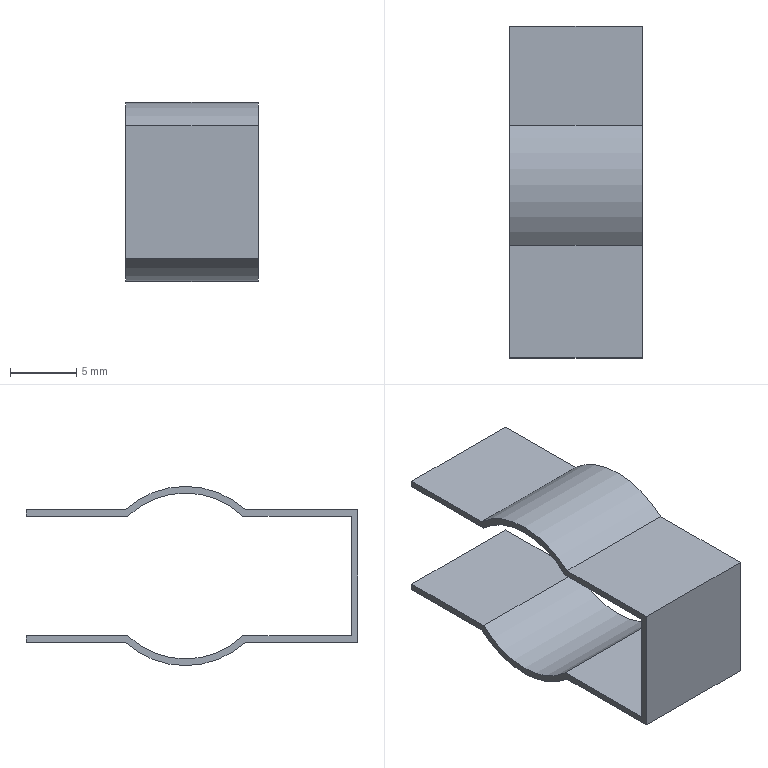Part | STEP file | 09-01 Heating tube seat | 1 solid | 18 faces | box 10 x 25 x 13.5 mm | volume 303.936 mm3 | plane 14 | cylinder 4 | commonest cylinder face diameters 12.5 x2 13.5 x2
STEP:
#1=CARTESIAN_POINT('',(0.,0.,0.));
#2=DIRECTION('',(0.,0.,1.));
#3=DIRECTION('',(1.,0.,0.));
#4=AXIS2_PLACEMENT_3D('',#1,#2,#3);
#5=CARTESIAN_POINT('',(5.,17.535,5.));
#6=VERTEX_POINT('',#5);
#7=CARTESIAN_POINT('',(5.,8.465,5.));
#8=VERTEX_POINT('',#7);
#9=CARTESIAN_POINT('',(5.,13.,0.));
#10=DIRECTION('',(1.,0.,0.));
#11=DIRECTION('',(0.,-1.,0.));
#12=AXIS2_PLACEMENT_3D('',#9,#10,#11);
#13=CIRCLE('',#12,6.75);
#14=CARTESIAN_POINT('',(5.,13.,0.));
#15=DIRECTION('',(-1.,0.,0.));
#16=DIRECTION('',(0.,-1.,0.));
#17=AXIS2_PLACEMENT_3D('',#14,#15,#16);
#18=CYLINDRICAL_SURFACE('',#17,6.75);
#19=CARTESIAN_POINT('',(6.283,0.));
#20=DIRECTION('',(-1.,0.));
#21=VECTOR('',#20,1.);
#22=LINE('',#19,#21);
#23=(GEOMETRIC_REPRESENTATION_CONTEXT(2)PARAMETRIC_REPRESENTATION_CONTEXT()REPRESENTATION_CONTEXT('',''));
#24=DEFINITIONAL_REPRESENTATION('',(#22),#23);
#25=PCURVE('',#18,#24);
#26=CARTESIAN_POINT('',(5.,0.,6.831));
#27=DIRECTION('',(1.,0.,0.));
#28=DIRECTION('',(0.,0.,-1.));
#29=AXIS2_PLACEMENT_3D('',#26,#27,#28);
#30=PLANE('',#29);
#31=CARTESIAN_POINT('',(6.831,13.));
#32=DIRECTION('',(0.,-1.));
#33=AXIS2_PLACEMENT_2D('',#31,#32);
#34=CIRCLE('',#33,6.75);
#35=(GEOMETRIC_REPRESENTATION_CONTEXT(2)PARAMETRIC_REPRESENTATION_CONTEXT()REPRESENTATION_CONTEXT('',''));
#36=DEFINITIONAL_REPRESENTATION('',(#34),#35);
#37=PCURVE('',#30,#36);
#38=SURFACE_CURVE('',#13,(#25,#37),.PCURVE_S1.);
#39=EDGE_CURVE('',#6,#8,#38,.T.);
#40=ORIENTED_EDGE('',*,*,#39,.F.);
#41=CARTESIAN_POINT('',(-5.,17.535,5.));
#42=VERTEX_POINT('',#41);
#43=CARTESIAN_POINT('',(0.,17.535,5.));
#44=DIRECTION('',(1.,0.,0.));
#45=VECTOR('',#44,1.);
#46=LINE('',#43,#45);
#47=CARTESIAN_POINT('',(2.307,5.));
#48=DIRECTION('',(0.,-1.));
#49=VECTOR('',#48,1.);
#50=LINE('',#47,#49);
#51=(GEOMETRIC_REPRESENTATION_CONTEXT(2)PARAMETRIC_REPRESENTATION_CONTEXT()REPRESENTATION_CONTEXT('',''));
#52=DEFINITIONAL_REPRESENTATION('',(#50),#51);
#53=PCURVE('',#18,#52);
#54=CARTESIAN_POINT('',(5.,17.535,5.));
#55=DIRECTION('',(0.,0.,-1.));
#56=DIRECTION('',(-1.,0.,0.));
#57=AXIS2_PLACEMENT_3D('',#54,#55,#56);
#58=PLANE('',#57);
#59=CARTESIAN_POINT('',(5.,0.));
#60=DIRECTION('',(-1.,0.));
#61=VECTOR('',#60,1.);
#62=LINE('',#59,#61);
#63=(GEOMETRIC_REPRESENTATION_CONTEXT(2)PARAMETRIC_REPRESENTATION_CONTEXT()REPRESENTATION_CONTEXT('',''));
#64=DEFINITIONAL_REPRESENTATION('',(#62),#63);
#65=PCURVE('',#58,#64);
#66=SURFACE_CURVE('',#46,(#53,#65),.PCURVE_S1.);
#67=EDGE_CURVE('',#42,#6,#66,.T.);
#68=ORIENTED_EDGE('',*,*,#67,.F.);
#69=CARTESIAN_POINT('',(-5.,8.465,5.));
#70=VERTEX_POINT('',#69);
#71=CARTESIAN_POINT('',(-5.,13.,0.));
#72=DIRECTION('',(-1.,0.,0.));
#73=DIRECTION('',(0.,-1.,0.));
#74=AXIS2_PLACEMENT_3D('',#71,#72,#73);
#75=CIRCLE('',#74,6.75);
#76=CARTESIAN_POINT('',(0.,10.));
#77=DIRECTION('',(1.,0.));
#78=VECTOR('',#77,1.);
#79=LINE('',#76,#78);
#80=(GEOMETRIC_REPRESENTATION_CONTEXT(2)PARAMETRIC_REPRESENTATION_CONTEXT()REPRESENTATION_CONTEXT('',''));
#81=DEFINITIONAL_REPRESENTATION('',(#79),#80);
#82=PCURVE('',#18,#81);
#83=CARTESIAN_POINT('',(-5.,0.,6.831));
#84=DIRECTION('',(1.,0.,0.));
#85=DIRECTION('',(0.,0.,-1.));
#86=AXIS2_PLACEMENT_3D('',#83,#84,#85);
#87=PLANE('',#86);
#88=CARTESIAN_POINT('',(6.831,6.25));
#89=CARTESIAN_POINT('',(-4.86,6.25));
#90=CARTESIAN_POINT('',(0.9853,16.375));
#91=CARTESIAN_POINT('',(6.831,26.5));
#92=CARTESIAN_POINT('',(12.677,16.375));
#93=CARTESIAN_POINT('',(18.522,6.25));
#94=CARTESIAN_POINT('',(6.831,6.25));
#95=(BOUNDED_CURVE()B_SPLINE_CURVE(2,(#88,#89,#90,#91,#92,#93,#94),.UNSPECIFIED.,.T.,.F.)B_SPLINE_CURVE_WITH_KNOTS((1,2,2,2,2,1),(-2.094,0.,2.094,4.189,6.283,8.378),.UNSPECIFIED.)CURVE()GEOMETRIC_REPRESENTATION_ITEM()RATIONAL_B_SPLINE_CURVE((1.,0.5,1.,0.5,1.,0.5,1.))REPRESENTATION_ITEM(''));
#96=(GEOMETRIC_REPRESENTATION_CONTEXT(2)PARAMETRIC_REPRESENTATION_CONTEXT()REPRESENTATION_CONTEXT('',''));
#97=DEFINITIONAL_REPRESENTATION('',(#95),#96);
#98=PCURVE('',#87,#97);
#99=SURFACE_CURVE('',#75,(#82,#98),.PCURVE_S1.);
#100=EDGE_CURVE('',#70,#42,#99,.T.);
#101=ORIENTED_EDGE('',*,*,#100,.F.);
#102=CARTESIAN_POINT('',(0.,8.465,5.));
#103=DIRECTION('',(-1.,0.,0.));
#104=VECTOR('',#103,1.);
#105=LINE('',#102,#104);
#106=CARTESIAN_POINT('',(0.8342,5.));
#107=DIRECTION('',(0.,1.));
#108=VECTOR('',#107,1.);
#109=LINE('',#106,#108);
#110=(GEOMETRIC_REPRESENTATION_CONTEXT(2)PARAMETRIC_REPRESENTATION_CONTEXT()REPRESENTATION_CONTEXT('',''));
#111=DEFINITIONAL_REPRESENTATION('',(#109),#110);
#112=PCURVE('',#18,#111);
#113=CARTESIAN_POINT('',(5.,0.,5.));
#114=DIRECTION('',(0.,0.,-1.));
#115=DIRECTION('',(-1.,0.,0.));
#116=AXIS2_PLACEMENT_3D('',#113,#114,#115);
#117=PLANE('',#116);
#118=CARTESIAN_POINT('',(5.,8.465));
#119=DIRECTION('',(1.,0.));
#120=VECTOR('',#119,1.);
#121=LINE('',#118,#120);
#122=(GEOMETRIC_REPRESENTATION_CONTEXT(2)PARAMETRIC_REPRESENTATION_CONTEXT()REPRESENTATION_CONTEXT('',''));
#123=DEFINITIONAL_REPRESENTATION('',(#121),#122);
#124=PCURVE('',#117,#123);
#125=SURFACE_CURVE('',#105,(#112,#124),.PCURVE_S1.);
#126=EDGE_CURVE('',#8,#70,#125,.T.);
#127=ORIENTED_EDGE('',*,*,#126,.F.);
#128=EDGE_LOOP('',(#40,#68,#101,#127));
#129=FACE_BOUND('',#128,.T.);
#130=ADVANCED_FACE('',(#129),#18,.T.);
#131=CARTESIAN_POINT('',(5.,25.,5.));
#132=VERTEX_POINT('',#131);
#133=CARTESIAN_POINT('',(5.,12.5,5.));
#134=DIRECTION('',(0.,-1.,0.));
#135=VECTOR('',#134,1.);
#136=LINE('',#133,#135);
#137=CARTESIAN_POINT('',(1.831,12.5));
#138=DIRECTION('',(0.,-1.));
#139=VECTOR('',#138,1.);
#140=LINE('',#137,#139);
#141=(GEOMETRIC_REPRESENTATION_CONTEXT(2)PARAMETRIC_REPRESENTATION_CONTEXT()REPRESENTATION_CONTEXT('',''));
#142=DEFINITIONAL_REPRESENTATION('',(#140),#141);
#143=PCURVE('',#30,#142);
#144=CARTESIAN_POINT('',(0.,-5.035));
#145=DIRECTION('',(0.,-1.));
#146=VECTOR('',#145,1.);
#147=LINE('',#144,#146);
#148=(GEOMETRIC_REPRESENTATION_CONTEXT(2)PARAMETRIC_REPRESENTATION_CONTEXT()REPRESENTATION_CONTEXT('',''));
#149=DEFINITIONAL_REPRESENTATION('',(#147),#148);
#150=PCURVE('',#58,#149);
#151=SURFACE_CURVE('',#136,(#143,#150),.PCURVE_S1.);
#152=EDGE_CURVE('',#132,#6,#151,.T.);
#153=ORIENTED_EDGE('',*,*,#152,.T.);
#154=ORIENTED_EDGE('',*,*,#39,.T.);
#155=CARTESIAN_POINT('',(5.,0.,5.));
#156=VERTEX_POINT('',#155);
#157=CARTESIAN_POINT('',(5.,12.5,5.));
#158=DIRECTION('',(0.,-1.,0.));
#159=VECTOR('',#158,1.);
#160=LINE('',#157,#159);
#161=CARTESIAN_POINT('',(1.831,12.5));
#162=DIRECTION('',(0.,-1.));
#163=VECTOR('',#162,1.);
#164=LINE('',#161,#163);
#165=(GEOMETRIC_REPRESENTATION_CONTEXT(2)PARAMETRIC_REPRESENTATION_CONTEXT()REPRESENTATION_CONTEXT('',''));
#166=DEFINITIONAL_REPRESENTATION('',(#164),#165);
#167=PCURVE('',#30,#166);
#168=CARTESIAN_POINT('',(0.,12.5));
#169=DIRECTION('',(0.,-1.));
#170=VECTOR('',#169,1.);
#171=LINE('',#168,#170);
#172=(GEOMETRIC_REPRESENTATION_CONTEXT(2)PARAMETRIC_REPRESENTATION_CONTEXT()REPRESENTATION_CONTEXT('',''));
#173=DEFINITIONAL_REPRESENTATION('',(#171),#172);
#174=PCURVE('',#117,#173);
#175=SURFACE_CURVE('',#160,(#167,#174),.PCURVE_S1.);
#176=EDGE_CURVE('',#8,#156,#175,.T.);
#177=ORIENTED_EDGE('',*,*,#176,.T.);
#178=CARTESIAN_POINT('',(5.,0.,-5.));
#179=VERTEX_POINT('',#178);
#180=CARTESIAN_POINT('',(5.,0.,0.));
#181=DIRECTION('',(0.,0.,-1.));
#182=VECTOR('',#181,1.);
#183=LINE('',#180,#182);
#184=CARTESIAN_POINT('',(6.831,0.));
#185=DIRECTION('',(1.,0.));
#186=VECTOR('',#185,1.);
#187=LINE('',#184,#186);
#188=(GEOMETRIC_REPRESENTATION_CONTEXT(2)PARAMETRIC_REPRESENTATION_CONTEXT()REPRESENTATION_CONTEXT('',''));
#189=DEFINITIONAL_REPRESENTATION('',(#187),#188);
#190=PCURVE('',#30,#189);
#191=CARTESIAN_POINT('',(-5.,0.,-5.));
#192=DIRECTION('',(0.,1.,0.));
#193=DIRECTION('',(0.,0.,1.));
#194=AXIS2_PLACEMENT_3D('',#191,#192,#193);
#195=PLANE('',#194);
#196=CARTESIAN_POINT('',(5.,10.));
#197=DIRECTION('',(-1.,0.));
#198=VECTOR('',#197,1.);
#199=LINE('',#196,#198);
#200=(GEOMETRIC_REPRESENTATION_CONTEXT(2)PARAMETRIC_REPRESENTATION_CONTEXT()REPRESENTATION_CONTEXT('',''));
#201=DEFINITIONAL_REPRESENTATION('',(#199),#200);
#202=PCURVE('',#195,#201);
#203=SURFACE_CURVE('',#183,(#190,#202),.PCURVE_S1.);
#204=EDGE_CURVE('',#156,#179,#203,.T.);
#205=ORIENTED_EDGE('',*,*,#204,.T.);
#206=CARTESIAN_POINT('',(5.,8.465,-5.));
#207=VERTEX_POINT('',#206);
#208=CARTESIAN_POINT('',(5.,12.5,-5.));
#209=DIRECTION('',(0.,1.,0.));
#210=VECTOR('',#209,1.);
#211=LINE('',#208,#210);
#212=CARTESIAN_POINT('',(11.831,12.5));
#213=DIRECTION('',(0.,1.));
#214=VECTOR('',#213,1.);
#215=LINE('',#212,#214);
#216=(GEOMETRIC_REPRESENTATION_CONTEXT(2)PARAMETRIC_REPRESENTATION_CONTEXT()REPRESENTATION_CONTEXT('',''));
#217=DEFINITIONAL_REPRESENTATION('',(#215),#216);
#218=PCURVE('',#30,#217);
#219=CARTESIAN_POINT('',(-5.,0.,-5.));
#220=DIRECTION('',(0.,0.,1.));
#221=DIRECTION('',(1.,0.,0.));
#222=AXIS2_PLACEMENT_3D('',#219,#220,#221);
#223=PLANE('',#222);
#224=CARTESIAN_POINT('',(10.,12.5));
#225=DIRECTION('',(0.,1.));
#226=VECTOR('',#225,1.);
#227=LINE('',#224,#226);
#228=(GEOMETRIC_REPRESENTATION_CONTEXT(2)PARAMETRIC_REPRESENTATION_CONTEXT()REPRESENTATION_CONTEXT('',''));
#229=DEFINITIONAL_REPRESENTATION('',(#227),#228);
#230=PCURVE('',#223,#229);
#231=SURFACE_CURVE('',#211,(#218,#230),.PCURVE_S1.);
#232=EDGE_CURVE('',#179,#207,#231,.T.);
#233=ORIENTED_EDGE('',*,*,#232,.T.);
#234=CARTESIAN_POINT('',(5.,17.535,-5.));
#235=VERTEX_POINT('',#234);
#236=CARTESIAN_POINT('',(5.,13.,0.));
#237=DIRECTION('',(1.,0.,0.));
#238=DIRECTION('',(0.,-1.,0.));
#239=AXIS2_PLACEMENT_3D('',#236,#237,#238);
#240=CIRCLE('',#239,6.75);
#241=CARTESIAN_POINT('',(6.831,13.));
#242=DIRECTION('',(0.,-1.));
#243=AXIS2_PLACEMENT_2D('',#241,#242);
#244=CIRCLE('',#243,6.75);
#245=(GEOMETRIC_REPRESENTATION_CONTEXT(2)PARAMETRIC_REPRESENTATION_CONTEXT()REPRESENTATION_CONTEXT('',''));
#246=DEFINITIONAL_REPRESENTATION('',(#244),#245);
#247=PCURVE('',#30,#246);
#248=CARTESIAN_POINT('',(5.,13.,0.));
#249=DIRECTION('',(-1.,0.,0.));
#250=DIRECTION('',(0.,-1.,0.));
#251=AXIS2_PLACEMENT_3D('',#248,#249,#250);
#252=CYLINDRICAL_SURFACE('',#251,6.75);
#253=CARTESIAN_POINT('',(6.283,0.));
#254=DIRECTION('',(-1.,0.));
#255=VECTOR('',#254,1.);
#256=LINE('',#253,#255);
#257=(GEOMETRIC_REPRESENTATION_CONTEXT(2)PARAMETRIC_REPRESENTATION_CONTEXT()REPRESENTATION_CONTEXT('',''));
#258=DEFINITIONAL_REPRESENTATION('',(#256),#257);
#259=PCURVE('',#252,#258);
#260=SURFACE_CURVE('',#240,(#247,#259),.PCURVE_S1.);
#261=EDGE_CURVE('',#207,#235,#260,.T.);
#262=ORIENTED_EDGE('',*,*,#261,.T.);
#263=CARTESIAN_POINT('',(5.,25.,-5.));
#264=VERTEX_POINT('',#263);
#265=CARTESIAN_POINT('',(5.,12.5,-5.));
#266=DIRECTION('',(0.,1.,0.));
#267=VECTOR('',#266,1.);
#268=LINE('',#265,#267);
#269=CARTESIAN_POINT('',(11.831,12.5));
#270=DIRECTION('',(0.,1.));
#271=VECTOR('',#270,1.);
#272=LINE('',#269,#271);
#273=(GEOMETRIC_REPRESENTATION_CONTEXT(2)PARAMETRIC_REPRESENTATION_CONTEXT()REPRESENTATION_CONTEXT('',''));
#274=DEFINITIONAL_REPRESENTATION('',(#272),#273);
#275=PCURVE('',#30,#274);
#276=CARTESIAN_POINT('',(-5.,25.,-5.));
#277=DIRECTION('',(0.,0.,1.));
#278=DIRECTION('',(0.,-1.,0.));
#279=AXIS2_PLACEMENT_3D('',#276,#277,#278);
#280=PLANE('',#279);
#281=CARTESIAN_POINT('',(12.5,10.));
#282=DIRECTION('',(-1.,0.));
#283=VECTOR('',#282,1.);
#284=LINE('',#281,#283);
#285=(GEOMETRIC_REPRESENTATION_CONTEXT(2)PARAMETRIC_REPRESENTATION_CONTEXT()REPRESENTATION_CONTEXT('',''));
#286=DEFINITIONAL_REPRESENTATION('',(#284),#285);
#287=PCURVE('',#280,#286);
#288=SURFACE_CURVE('',#268,(#275,#287),.PCURVE_S1.);
#289=EDGE_CURVE('',#235,#264,#288,.T.);
#290=ORIENTED_EDGE('',*,*,#289,.T.);
#291=CARTESIAN_POINT('',(5.,25.,-4.5));
#292=VERTEX_POINT('',#291);
#293=CARTESIAN_POINT('',(5.,25.,-4.75));
#294=DIRECTION('',(0.,0.,1.));
#295=VECTOR('',#294,1.);
#296=LINE('',#293,#295);
#297=CARTESIAN_POINT('',(11.581,25.));
#298=DIRECTION('',(-1.,0.));
#299=VECTOR('',#298,1.);
#300=LINE('',#297,#299);
#301=(GEOMETRIC_REPRESENTATION_CONTEXT(2)PARAMETRIC_REPRESENTATION_CONTEXT()REPRESENTATION_CONTEXT('',''));
#302=DEFINITIONAL_REPRESENTATION('',(#300),#301);
#303=PCURVE('',#30,#302);
#304=CARTESIAN_POINT('',(-5.,25.,-4.5));
#305=DIRECTION('',(0.,-1.,0.));
#306=DIRECTION('',(0.,0.,-1.));
#307=AXIS2_PLACEMENT_3D('',#304,#305,#306);
#308=PLANE('',#307);
#309=CARTESIAN_POINT('',(0.25,10.));
#310=DIRECTION('',(-1.,0.));
#311=VECTOR('',#310,1.);
#312=LINE('',#309,#311);
#313=(GEOMETRIC_REPRESENTATION_CONTEXT(2)PARAMETRIC_REPRESENTATION_CONTEXT()REPRESENTATION_CONTEXT('',''));
#314=DEFINITIONAL_REPRESENTATION('',(#312),#313);
#315=PCURVE('',#308,#314);
#316=SURFACE_CURVE('',#296,(#303,#315),.PCURVE_S1.);
#317=EDGE_CURVE('',#264,#292,#316,.T.);
#318=ORIENTED_EDGE('',*,*,#317,.T.);
#319=CARTESIAN_POINT('',(5.,17.337,-4.5));
#320=VERTEX_POINT('',#319);
#321=CARTESIAN_POINT('',(5.,12.5,-4.5));
#322=DIRECTION('',(0.,-1.,0.));
#323=VECTOR('',#322,1.);
#324=LINE('',#321,#323);
#325=CARTESIAN_POINT('',(11.331,12.5));
#326=DIRECTION('',(0.,-1.));
#327=VECTOR('',#326,1.);
#328=LINE('',#325,#327);
#329=(GEOMETRIC_REPRESENTATION_CONTEXT(2)PARAMETRIC_REPRESENTATION_CONTEXT()REPRESENTATION_CONTEXT('',''));
#330=DEFINITIONAL_REPRESENTATION('',(#328),#329);
#331=PCURVE('',#30,#330);
#332=CARTESIAN_POINT('',(5.,17.337,-4.5));
#333=DIRECTION('',(0.,0.,-1.));
#334=DIRECTION('',(-1.,0.,0.));
#335=AXIS2_PLACEMENT_3D('',#332,#333,#334);
#336=PLANE('',#335);
#337=CARTESIAN_POINT('',(0.,-4.837));
#338=DIRECTION('',(0.,-1.));
#339=VECTOR('',#338,1.);
#340=LINE('',#337,#339);
#341=(GEOMETRIC_REPRESENTATION_CONTEXT(2)PARAMETRIC_REPRESENTATION_CONTEXT()REPRESENTATION_CONTEXT('',''));
#342=DEFINITIONAL_REPRESENTATION('',(#340),#341);
#343=PCURVE('',#336,#342);
#344=SURFACE_CURVE('',#324,(#331,#343),.PCURVE_S1.);
#345=EDGE_CURVE('',#292,#320,#344,.T.);
#346=ORIENTED_EDGE('',*,*,#345,.T.);
#347=CARTESIAN_POINT('',(5.,8.663,-4.5));
#348=VERTEX_POINT('',#347);
#349=CARTESIAN_POINT('',(5.,13.,0.));
#350=DIRECTION('',(-1.,0.,0.));
#351=DIRECTION('',(0.,-1.,0.));
#352=AXIS2_PLACEMENT_3D('',#349,#350,#351);
#353=CIRCLE('',#352,6.25);
#354=CARTESIAN_POINT('',(6.831,6.75));
#355=CARTESIAN_POINT('',(-3.994,6.75));
#356=CARTESIAN_POINT('',(1.418,16.125));
#357=CARTESIAN_POINT('',(6.831,25.5));
#358=CARTESIAN_POINT('',(12.244,16.125));
#359=CARTESIAN_POINT('',(17.656,6.75));
#360=CARTESIAN_POINT('',(6.831,6.75));
#361=(BOUNDED_CURVE()B_SPLINE_CURVE(2,(#354,#355,#356,#357,#358,#359,#360),.UNSPECIFIED.,.T.,.F.)B_SPLINE_CURVE_WITH_KNOTS((1,2,2,2,2,1),(-2.094,0.,2.094,4.189,6.283,8.378),.UNSPECIFIED.)CURVE()GEOMETRIC_REPRESENTATION_ITEM()RATIONAL_B_SPLINE_CURVE((1.,0.5,1.,0.5,1.,0.5,1.))REPRESENTATION_ITEM(''));
#362=(GEOMETRIC_REPRESENTATION_CONTEXT(2)PARAMETRIC_REPRESENTATION_CONTEXT()REPRESENTATION_CONTEXT('',''));
#363=DEFINITIONAL_REPRESENTATION('',(#361),#362);
#364=PCURVE('',#30,#363);
#365=CARTESIAN_POINT('',(5.,13.,0.));
#366=DIRECTION('',(-1.,0.,0.));
#367=DIRECTION('',(0.,-1.,0.));
#368=AXIS2_PLACEMENT_3D('',#365,#366,#367);
#369=CYLINDRICAL_SURFACE('',#368,6.25);
#370=CARTESIAN_POINT('',(0.,0.));
#371=DIRECTION('',(1.,0.));
#372=VECTOR('',#371,1.);
#373=LINE('',#370,#372);
#374=(GEOMETRIC_REPRESENTATION_CONTEXT(2)PARAMETRIC_REPRESENTATION_CONTEXT()REPRESENTATION_CONTEXT('',''));
#375=DEFINITIONAL_REPRESENTATION('',(#373),#374);
#376=PCURVE('',#369,#375);
#377=SURFACE_CURVE('',#353,(#364,#376),.PCURVE_S1.);
#378=EDGE_CURVE('',#320,#348,#377,.T.);
#379=ORIENTED_EDGE('',*,*,#378,.T.);
#380=CARTESIAN_POINT('',(5.,0.5,-4.5));
#381=VERTEX_POINT('',#380);
#382=CARTESIAN_POINT('',(5.,12.5,-4.5));
#383=DIRECTION('',(0.,-1.,0.));
#384=VECTOR('',#383,1.);
#385=LINE('',#382,#384);
#386=CARTESIAN_POINT('',(11.331,12.5));
#387=DIRECTION('',(0.,-1.));
#388=VECTOR('',#387,1.);
#389=LINE('',#386,#388);
#390=(GEOMETRIC_REPRESENTATION_CONTEXT(2)PARAMETRIC_REPRESENTATION_CONTEXT()REPRESENTATION_CONTEXT('',''));
#391=DEFINITIONAL_REPRESENTATION('',(#389),#390);
#392=PCURVE('',#30,#391);
#393=CARTESIAN_POINT('',(-5.,0.5,-4.5));
#394=DIRECTION('',(0.,0.,-1.));
#395=DIRECTION('',(0.,1.,0.));
#396=AXIS2_PLACEMENT_3D('',#393,#394,#395);
#397=PLANE('',#396);
#398=CARTESIAN_POINT('',(12.,10.));
#399=DIRECTION('',(-1.,0.));
#400=VECTOR('',#399,1.);
#401=LINE('',#398,#400);
#402=(GEOMETRIC_REPRESENTATION_CONTEXT(2)PARAMETRIC_REPRESENTATION_CONTEXT()REPRESENTATION_CONTEXT('',''));
#403=DEFINITIONAL_REPRESENTATION('',(#401),#402);
#404=PCURVE('',#397,#403);
#405=SURFACE_CURVE('',#385,(#392,#404),.PCURVE_S1.);
#406=EDGE_CURVE('',#348,#381,#405,.T.);
#407=ORIENTED_EDGE('',*,*,#406,.T.);
#408=CARTESIAN_POINT('',(5.,0.5,4.5));
#409=VERTEX_POINT('',#408);
#410=CARTESIAN_POINT('',(5.,0.5,0.));
#411=DIRECTION('',(0.,0.,1.));
#412=VECTOR('',#411,1.);
#413=LINE('',#410,#412);
#414=CARTESIAN_POINT('',(6.831,0.5));
#415=DIRECTION('',(-1.,0.));
#416=VECTOR('',#415,1.);
#417=LINE('',#414,#416);
#418=(GEOMETRIC_REPRESENTATION_CONTEXT(2)PARAMETRIC_REPRESENTATION_CONTEXT()REPRESENTATION_CONTEXT('',''));
#419=DEFINITIONAL_REPRESENTATION('',(#417),#418);
#420=PCURVE('',#30,#419);
#421=CARTESIAN_POINT('',(-5.,0.5,4.5));
#422=DIRECTION('',(0.,-1.,0.));
#423=DIRECTION('',(0.,0.,-1.));
#424=AXIS2_PLACEMENT_3D('',#421,#422,#423);
#425=PLANE('',#424);
#426=CARTESIAN_POINT('',(4.5,10.));
#427=DIRECTION('',(-1.,0.));
#428=VECTOR('',#427,1.);
#429=LINE('',#426,#428);
#430=(GEOMETRIC_REPRESENTATION_CONTEXT(2)PARAMETRIC_REPRESENTATION_CONTEXT()REPRESENTATION_CONTEXT('',''));
#431=DEFINITIONAL_REPRESENTATION('',(#429),#430);
#432=PCURVE('',#425,#431);
#433=SURFACE_CURVE('',#413,(#420,#432),.PCURVE_S1.);
#434=EDGE_CURVE('',#381,#409,#433,.T.);
#435=ORIENTED_EDGE('',*,*,#434,.T.);
#436=CARTESIAN_POINT('',(5.,8.663,4.5));
#437=VERTEX_POINT('',#436);
#438=CARTESIAN_POINT('',(5.,12.5,4.5));
#439=DIRECTION('',(0.,1.,0.));
#440=VECTOR('',#439,1.);
#441=LINE('',#438,#440);
#442=CARTESIAN_POINT('',(2.331,12.5));
#443=DIRECTION('',(0.,1.));
#444=VECTOR('',#443,1.);
#445=LINE('',#442,#444);
#446=(GEOMETRIC_REPRESENTATION_CONTEXT(2)PARAMETRIC_REPRESENTATION_CONTEXT()REPRESENTATION_CONTEXT('',''));
#447=DEFINITIONAL_REPRESENTATION('',(#445),#446);
#448=PCURVE('',#30,#447);
#449=CARTESIAN_POINT('',(-5.,0.5,4.5));
#450=DIRECTION('',(0.,0.,1.));
#451=DIRECTION('',(1.,0.,0.));
#452=AXIS2_PLACEMENT_3D('',#449,#450,#451);
#453=PLANE('',#452);
#454=CARTESIAN_POINT('',(10.,12.));
#455=DIRECTION('',(0.,1.));
#456=VECTOR('',#455,1.);
#457=LINE('',#454,#456);
#458=(GEOMETRIC_REPRESENTATION_CONTEXT(2)PARAMETRIC_REPRESENTATION_CONTEXT()REPRESENTATION_CONTEXT('',''));
#459=DEFINITIONAL_REPRESENTATION('',(#457),#458);
#460=PCURVE('',#453,#459);
#461=SURFACE_CURVE('',#441,(#448,#460),.PCURVE_S1.);
#462=EDGE_CURVE('',#409,#437,#461,.T.);
#463=ORIENTED_EDGE('',*,*,#462,.T.);
#464=CARTESIAN_POINT('',(5.,17.337,4.5));
#465=VERTEX_POINT('',#464);
#466=CARTESIAN_POINT('',(5.,13.,0.));
#467=DIRECTION('',(-1.,0.,0.));
#468=DIRECTION('',(0.,-1.,0.));
#469=AXIS2_PLACEMENT_3D('',#466,#467,#468);
#470=CIRCLE('',#469,6.25);
#471=CARTESIAN_POINT('',(6.831,6.75));
#472=CARTESIAN_POINT('',(-3.994,6.75));
#473=CARTESIAN_POINT('',(1.418,16.125));
#474=CARTESIAN_POINT('',(6.831,25.5));
#475=CARTESIAN_POINT('',(12.244,16.125));
#476=CARTESIAN_POINT('',(17.656,6.75));
#477=CARTESIAN_POINT('',(6.831,6.75));
#478=(BOUNDED_CURVE()B_SPLINE_CURVE(2,(#471,#472,#473,#474,#475,#476,#477),.UNSPECIFIED.,.T.,.F.)B_SPLINE_CURVE_WITH_KNOTS((1,2,2,2,2,1),(-2.094,0.,2.094,4.189,6.283,8.378),.UNSPECIFIED.)CURVE()GEOMETRIC_REPRESENTATION_ITEM()RATIONAL_B_SPLINE_CURVE((1.,0.5,1.,0.5,1.,0.5,1.))REPRESENTATION_ITEM(''));
#479=(GEOMETRIC_REPRESENTATION_CONTEXT(2)PARAMETRIC_REPRESENTATION_CONTEXT()REPRESENTATION_CONTEXT('',''));
#480=DEFINITIONAL_REPRESENTATION('',(#478),#479);
#481=PCURVE('',#30,#480);
#482=CARTESIAN_POINT('',(5.,13.,0.));
#483=DIRECTION('',(-1.,0.,0.));
#484=DIRECTION('',(0.,-1.,0.));
#485=AXIS2_PLACEMENT_3D('',#482,#483,#484);
#486=CYLINDRICAL_SURFACE('',#485,6.25);
#487=CARTESIAN_POINT('',(0.,0.));
#488=DIRECTION('',(1.,0.));
#489=VECTOR('',#488,1.);
#490=LINE('',#487,#489);
#491=(GEOMETRIC_REPRESENTATION_CONTEXT(2)PARAMETRIC_REPRESENTATION_CONTEXT()REPRESENTATION_CONTEXT('',''));
#492=DEFINITIONAL_REPRESENTATION('',(#490),#491);
#493=PCURVE('',#486,#492);
#494=SURFACE_CURVE('',#470,(#481,#493),.PCURVE_S1.);
#495=EDGE_CURVE('',#437,#465,#494,.T.);
#496=ORIENTED_EDGE('',*,*,#495,.T.);
#497=CARTESIAN_POINT('',(5.,25.,4.5));
#498=VERTEX_POINT('',#497);
#499=CARTESIAN_POINT('',(5.,12.5,4.5));
#500=DIRECTION('',(0.,1.,0.));
#501=VECTOR('',#500,1.);
#502=LINE('',#499,#501);
#503=CARTESIAN_POINT('',(2.331,12.5));
#504=DIRECTION('',(0.,1.));
#505=VECTOR('',#504,1.);
#506=LINE('',#503,#505);
#507=(GEOMETRIC_REPRESENTATION_CONTEXT(2)PARAMETRIC_REPRESENTATION_CONTEXT()REPRESENTATION_CONTEXT('',''));
#508=DEFINITIONAL_REPRESENTATION('',(#506),#507);
#509=PCURVE('',#30,#508);
#510=CARTESIAN_POINT('',(-5.,17.337,4.5));
#511=DIRECTION('',(0.,0.,1.));
#512=DIRECTION('',(1.,0.,0.));
#513=AXIS2_PLACEMENT_3D('',#510,#511,#512);
#514=PLANE('',#513);
#515=CARTESIAN_POINT('',(10.,-4.837));
#516=DIRECTION('',(0.,1.));
#517=VECTOR('',#516,1.);
#518=LINE('',#515,#517);
#519=(GEOMETRIC_REPRESENTATION_CONTEXT(2)PARAMETRIC_REPRESENTATION_CONTEXT()REPRESENTATION_CONTEXT('',''));
#520=DEFINITIONAL_REPRESENTATION('',(#518),#519);
#521=PCURVE('',#514,#520);
#522=SURFACE_CURVE('',#502,(#509,#521),.PCURVE_S1.);
#523=EDGE_CURVE('',#465,#498,#522,.T.);
#524=ORIENTED_EDGE('',*,*,#523,.T.);
#525=CARTESIAN_POINT('',(5.,25.,4.75));
#526=DIRECTION('',(0.,0.,1.));
#527=VECTOR('',#526,1.);
#528=LINE('',#525,#527);
#529=CARTESIAN_POINT('',(2.081,25.));
#530=DIRECTION('',(-1.,0.));
#531=VECTOR('',#530,1.);
#532=LINE('',#529,#531);
#533=(GEOMETRIC_REPRESENTATION_CONTEXT(2)PARAMETRIC_REPRESENTATION_CONTEXT()REPRESENTATION_CONTEXT('',''));
#534=DEFINITIONAL_REPRESENTATION('',(#532),#533);
#535=PCURVE('',#30,#534);
#536=CARTESIAN_POINT('',(-5.,25.,5.));
#537=DIRECTION('',(0.,-1.,0.));
#538=DIRECTION('',(0.,0.,-1.));
#539=AXIS2_PLACEMENT_3D('',#536,#537,#538);
#540=PLANE('',#539);
#541=CARTESIAN_POINT('',(0.25,10.));
#542=DIRECTION('',(-1.,0.));
#543=VECTOR('',#542,1.);
#544=LINE('',#541,#543);
#545=(GEOMETRIC_REPRESENTATION_CONTEXT(2)PARAMETRIC_REPRESENTATION_CONTEXT()REPRESENTATION_CONTEXT('',''));
#546=DEFINITIONAL_REPRESENTATION('',(#544),#545);
#547=PCURVE('',#540,#546);
#548=SURFACE_CURVE('',#528,(#535,#547),.PCURVE_S1.);
#549=EDGE_CURVE('',#498,#132,#548,.T.);
#550=ORIENTED_EDGE('',*,*,#549,.T.);
#551=EDGE_LOOP('',(#153,#154,#177,#205,#233,#262,#290,#318,#346,#379,#407,#435,#463,#496,#524,#550));
#552=FACE_BOUND('',#551,.T.);
#553=ADVANCED_FACE('',(#552),#30,.T.);
#554=ORIENTED_EDGE('',*,*,#100,.T.);
#555=CARTESIAN_POINT('',(-5.,25.,5.));
#556=VERTEX_POINT('',#555);
#557=CARTESIAN_POINT('',(-5.,12.5,5.));
#558=DIRECTION('',(0.,-1.,0.));
#559=VECTOR('',#558,1.);
#560=LINE('',#557,#559);
#561=CARTESIAN_POINT('',(1.831,12.5));
#562=DIRECTION('',(0.,-1.));
#563=VECTOR('',#562,1.);
#564=LINE('',#561,#563);
#565=(GEOMETRIC_REPRESENTATION_CONTEXT(2)PARAMETRIC_REPRESENTATION_CONTEXT()REPRESENTATION_CONTEXT('',''));
#566=DEFINITIONAL_REPRESENTATION('',(#564),#565);
#567=PCURVE('',#87,#566);
#568=CARTESIAN_POINT('',(10.,-5.035));
#569=DIRECTION('',(0.,-1.));
#570=VECTOR('',#569,1.);
#571=LINE('',#568,#570);
#572=(GEOMETRIC_REPRESENTATION_CONTEXT(2)PARAMETRIC_REPRESENTATION_CONTEXT()REPRESENTATION_CONTEXT('',''));
#573=DEFINITIONAL_REPRESENTATION('',(#571),#572);
#574=PCURVE('',#58,#573);
#575=SURFACE_CURVE('',#560,(#567,#574),.PCURVE_S1.);
#576=EDGE_CURVE('',#556,#42,#575,.T.);
#577=ORIENTED_EDGE('',*,*,#576,.F.);
#578=CARTESIAN_POINT('',(-5.,25.,4.5));
#579=VERTEX_POINT('',#578);
#580=CARTESIAN_POINT('',(-5.,25.,4.75));
#581=DIRECTION('',(0.,0.,-1.));
#582=VECTOR('',#581,1.);
#583=LINE('',#580,#582);
#584=CARTESIAN_POINT('',(2.081,25.));
#585=DIRECTION('',(1.,0.));
#586=VECTOR('',#585,1.);
#587=LINE('',#584,#586);
#588=(GEOMETRIC_REPRESENTATION_CONTEXT(2)PARAMETRIC_REPRESENTATION_CONTEXT()REPRESENTATION_CONTEXT('',''));
#589=DEFINITIONAL_REPRESENTATION('',(#587),#588);
#590=PCURVE('',#87,#589);
#591=CARTESIAN_POINT('',(0.25,0.));
#592=DIRECTION('',(1.,0.));
#593=VECTOR('',#592,1.);
#594=LINE('',#591,#593);
#595=(GEOMETRIC_REPRESENTATION_CONTEXT(2)PARAMETRIC_REPRESENTATION_CONTEXT()REPRESENTATION_CONTEXT('',''));
#596=DEFINITIONAL_REPRESENTATION('',(#594),#595);
#597=PCURVE('',#540,#596);
#598=SURFACE_CURVE('',#583,(#590,#597),.PCURVE_S1.);
#599=EDGE_CURVE('',#556,#579,#598,.T.);
#600=ORIENTED_EDGE('',*,*,#599,.T.);
#601=CARTESIAN_POINT('',(-5.,17.337,4.5));
#602=VERTEX_POINT('',#601);
#603=CARTESIAN_POINT('',(-5.,12.5,4.5));
#604=DIRECTION('',(0.,1.,0.));
#605=VECTOR('',#604,1.);
#606=LINE('',#603,#605);
#607=CARTESIAN_POINT('',(2.331,12.5));
#608=DIRECTION('',(0.,1.));
#609=VECTOR('',#608,1.);
#610=LINE('',#607,#609);
#611=(GEOMETRIC_REPRESENTATION_CONTEXT(2)PARAMETRIC_REPRESENTATION_CONTEXT()REPRESENTATION_CONTEXT('',''));
#612=DEFINITIONAL_REPRESENTATION('',(#610),#611);
#613=PCURVE('',#87,#612);
#614=CARTESIAN_POINT('',(0.,-4.837));
#615=DIRECTION('',(0.,1.));
#616=VECTOR('',#615,1.);
#617=LINE('',#614,#616);
#618=(GEOMETRIC_REPRESENTATION_CONTEXT(2)PARAMETRIC_REPRESENTATION_CONTEXT()REPRESENTATION_CONTEXT('',''));
#619=DEFINITIONAL_REPRESENTATION('',(#617),#618);
#620=PCURVE('',#514,#619);
#621=SURFACE_CURVE('',#606,(#613,#620),.PCURVE_S1.);
#622=EDGE_CURVE('',#602,#579,#621,.T.);
#623=ORIENTED_EDGE('',*,*,#622,.F.);
#624=CARTESIAN_POINT('',(-5.,8.663,4.5));
#625=VERTEX_POINT('',#624);
#626=CARTESIAN_POINT('',(-5.,13.,0.));
#627=DIRECTION('',(-1.,0.,0.));
#628=DIRECTION('',(0.,-1.,0.));
#629=AXIS2_PLACEMENT_3D('',#626,#627,#628);
#630=CIRCLE('',#629,6.25);
#631=CARTESIAN_POINT('',(6.831,6.75));
#632=CARTESIAN_POINT('',(-3.994,6.75));
#633=CARTESIAN_POINT('',(1.418,16.125));
#634=CARTESIAN_POINT('',(6.831,25.5));
#635=CARTESIAN_POINT('',(12.244,16.125));
#636=CARTESIAN_POINT('',(17.656,6.75));
#637=CARTESIAN_POINT('',(6.831,6.75));
#638=(BOUNDED_CURVE()B_SPLINE_CURVE(2,(#631,#632,#633,#634,#635,#636,#637),.UNSPECIFIED.,.T.,.F.)B_SPLINE_CURVE_WITH_KNOTS((1,2,2,2,2,1),(-2.094,0.,2.094,4.189,6.283,8.378),.UNSPECIFIED.)CURVE()GEOMETRIC_REPRESENTATION_ITEM()RATIONAL_B_SPLINE_CURVE((1.,0.5,1.,0.5,1.,0.5,1.))REPRESENTATION_ITEM(''));
#639=(GEOMETRIC_REPRESENTATION_CONTEXT(2)PARAMETRIC_REPRESENTATION_CONTEXT()REPRESENTATION_CONTEXT('',''));
#640=DEFINITIONAL_REPRESENTATION('',(#638),#639);
#641=PCURVE('',#87,#640);
#642=CARTESIAN_POINT('',(0.,10.));
#643=DIRECTION('',(1.,0.));
#644=VECTOR('',#643,1.);
#645=LINE('',#642,#644);
#646=(GEOMETRIC_REPRESENTATION_CONTEXT(2)PARAMETRIC_REPRESENTATION_CONTEXT()REPRESENTATION_CONTEXT('',''));
#647=DEFINITIONAL_REPRESENTATION('',(#645),#646);
#648=PCURVE('',#486,#647);
#649=SURFACE_CURVE('',#630,(#641,#648),.PCURVE_S1.);
#650=EDGE_CURVE('',#625,#602,#649,.T.);
#651=ORIENTED_EDGE('',*,*,#650,.F.);
#652=CARTESIAN_POINT('',(-5.,0.5,4.5));
#653=VERTEX_POINT('',#652);
#654=CARTESIAN_POINT('',(-5.,12.5,4.5));
#655=DIRECTION('',(0.,1.,0.));
#656=VECTOR('',#655,1.);
#657=LINE('',#654,#656);
#658=CARTESIAN_POINT('',(2.331,12.5));
#659=DIRECTION('',(0.,1.));
#660=VECTOR('',#659,1.);
#661=LINE('',#658,#660);
#662=(GEOMETRIC_REPRESENTATION_CONTEXT(2)PARAMETRIC_REPRESENTATION_CONTEXT()REPRESENTATION_CONTEXT('',''));
#663=DEFINITIONAL_REPRESENTATION('',(#661),#662);
#664=PCURVE('',#87,#663);
#665=CARTESIAN_POINT('',(0.,12.));
#666=DIRECTION('',(0.,1.));
#667=VECTOR('',#666,1.);
#668=LINE('',#665,#667);
#669=(GEOMETRIC_REPRESENTATION_CONTEXT(2)PARAMETRIC_REPRESENTATION_CONTEXT()REPRESENTATION_CONTEXT('',''));
#670=DEFINITIONAL_REPRESENTATION('',(#668),#669);
#671=PCURVE('',#453,#670);
#672=SURFACE_CURVE('',#657,(#664,#671),.PCURVE_S1.);
#673=EDGE_CURVE('',#653,#625,#672,.T.);
#674=ORIENTED_EDGE('',*,*,#673,.F.);
#675=CARTESIAN_POINT('',(-5.,0.5,-4.5));
#676=VERTEX_POINT('',#675);
#677=CARTESIAN_POINT('',(-5.,0.5,0.));
#678=DIRECTION('',(0.,0.,1.));
#679=VECTOR('',#678,1.);
#680=LINE('',#677,#679);
#681=CARTESIAN_POINT('',(6.831,0.5));
#682=DIRECTION('',(-1.,0.));
#683=VECTOR('',#682,1.);
#684=LINE('',#681,#683);
#685=(GEOMETRIC_REPRESENTATION_CONTEXT(2)PARAMETRIC_REPRESENTATION_CONTEXT()REPRESENTATION_CONTEXT('',''));
#686=DEFINITIONAL_REPRESENTATION('',(#684),#685);
#687=PCURVE('',#87,#686);
#688=CARTESIAN_POINT('',(4.5,0.));
#689=DIRECTION('',(-1.,0.));
#690=VECTOR('',#689,1.);
#691=LINE('',#688,#690);
#692=(GEOMETRIC_REPRESENTATION_CONTEXT(2)PARAMETRIC_REPRESENTATION_CONTEXT()REPRESENTATION_CONTEXT('',''));
#693=DEFINITIONAL_REPRESENTATION('',(#691),#692);
#694=PCURVE('',#425,#693);
#695=SURFACE_CURVE('',#680,(#687,#694),.PCURVE_S1.);
#696=EDGE_CURVE('',#676,#653,#695,.T.);
#697=ORIENTED_EDGE('',*,*,#696,.F.);
#698=CARTESIAN_POINT('',(-5.,8.663,-4.5));
#699=VERTEX_POINT('',#698);
#700=CARTESIAN_POINT('',(-5.,12.5,-4.5));
#701=DIRECTION('',(0.,-1.,0.));
#702=VECTOR('',#701,1.);
#703=LINE('',#700,#702);
#704=CARTESIAN_POINT('',(11.331,12.5));
#705=DIRECTION('',(0.,-1.));
#706=VECTOR('',#705,1.);
#707=LINE('',#704,#706);
#708=(GEOMETRIC_REPRESENTATION_CONTEXT(2)PARAMETRIC_REPRESENTATION_CONTEXT()REPRESENTATION_CONTEXT('',''));
#709=DEFINITIONAL_REPRESENTATION('',(#707),#708);
#710=PCURVE('',#87,#709);
#711=CARTESIAN_POINT('',(12.,0.));
#712=DIRECTION('',(-1.,0.));
#713=VECTOR('',#712,1.);
#714=LINE('',#711,#713);
#715=(GEOMETRIC_REPRESENTATION_CONTEXT(2)PARAMETRIC_REPRESENTATION_CONTEXT()REPRESENTATION_CONTEXT('',''));
#716=DEFINITIONAL_REPRESENTATION('',(#714),#715);
#717=PCURVE('',#397,#716);
#718=SURFACE_CURVE('',#703,(#710,#717),.PCURVE_S1.);
#719=EDGE_CURVE('',#699,#676,#718,.T.);
#720=ORIENTED_EDGE('',*,*,#719,.F.);
#721=CARTESIAN_POINT('',(-5.,17.337,-4.5));
#722=VERTEX_POINT('',#721);
#723=CARTESIAN_POINT('',(-5.,13.,0.));
#724=DIRECTION('',(-1.,0.,0.));
#725=DIRECTION('',(0.,-1.,0.));
#726=AXIS2_PLACEMENT_3D('',#723,#724,#725);
#727=CIRCLE('',#726,6.25);
#728=CARTESIAN_POINT('',(6.831,6.75));
#729=CARTESIAN_POINT('',(-3.994,6.75));
#730=CARTESIAN_POINT('',(1.418,16.125));
#731=CARTESIAN_POINT('',(6.831,25.5));
#732=CARTESIAN_POINT('',(12.244,16.125));
#733=CARTESIAN_POINT('',(17.656,6.75));
#734=CARTESIAN_POINT('',(6.831,6.75));
#735=(BOUNDED_CURVE()B_SPLINE_CURVE(2,(#728,#729,#730,#731,#732,#733,#734),.UNSPECIFIED.,.T.,.F.)B_SPLINE_CURVE_WITH_KNOTS((1,2,2,2,2,1),(-2.094,0.,2.094,4.189,6.283,8.378),.UNSPECIFIED.)CURVE()GEOMETRIC_REPRESENTATION_ITEM()RATIONAL_B_SPLINE_CURVE((1.,0.5,1.,0.5,1.,0.5,1.))REPRESENTATION_ITEM(''));
#736=(GEOMETRIC_REPRESENTATION_CONTEXT(2)PARAMETRIC_REPRESENTATION_CONTEXT()REPRESENTATION_CONTEXT('',''));
#737=DEFINITIONAL_REPRESENTATION('',(#735),#736);
#738=PCURVE('',#87,#737);
#739=CARTESIAN_POINT('',(0.,10.));
#740=DIRECTION('',(1.,0.));
#741=VECTOR('',#740,1.);
#742=LINE('',#739,#741);
#743=(GEOMETRIC_REPRESENTATION_CONTEXT(2)PARAMETRIC_REPRESENTATION_CONTEXT()REPRESENTATION_CONTEXT('',''));
#744=DEFINITIONAL_REPRESENTATION('',(#742),#743);
#745=PCURVE('',#369,#744);
#746=SURFACE_CURVE('',#727,(#738,#745),.PCURVE_S1.);
#747=EDGE_CURVE('',#722,#699,#746,.T.);
#748=ORIENTED_EDGE('',*,*,#747,.F.);
#749=CARTESIAN_POINT('',(-5.,25.,-4.5));
#750=VERTEX_POINT('',#749);
#751=CARTESIAN_POINT('',(-5.,12.5,-4.5));
#752=DIRECTION('',(0.,-1.,0.));
#753=VECTOR('',#752,1.);
#754=LINE('',#751,#753);
#755=CARTESIAN_POINT('',(11.331,12.5));
#756=DIRECTION('',(0.,-1.));
#757=VECTOR('',#756,1.);
#758=LINE('',#755,#757);
#759=(GEOMETRIC_REPRESENTATION_CONTEXT(2)PARAMETRIC_REPRESENTATION_CONTEXT()REPRESENTATION_CONTEXT('',''));
#760=DEFINITIONAL_REPRESENTATION('',(#758),#759);
#761=PCURVE('',#87,#760);
#762=CARTESIAN_POINT('',(10.,-4.837));
#763=DIRECTION('',(0.,-1.));
#764=VECTOR('',#763,1.);
#765=LINE('',#762,#764);
#766=(GEOMETRIC_REPRESENTATION_CONTEXT(2)PARAMETRIC_REPRESENTATION_CONTEXT()REPRESENTATION_CONTEXT('',''));
#767=DEFINITIONAL_REPRESENTATION('',(#765),#766);
#768=PCURVE('',#336,#767);
#769=SURFACE_CURVE('',#754,(#761,#768),.PCURVE_S1.);
#770=EDGE_CURVE('',#750,#722,#769,.T.);
#771=ORIENTED_EDGE('',*,*,#770,.F.);
#772=CARTESIAN_POINT('',(-5.,25.,-5.));
#773=VERTEX_POINT('',#772);
#774=CARTESIAN_POINT('',(-5.,25.,-4.75));
#775=DIRECTION('',(0.,0.,-1.));
#776=VECTOR('',#775,1.);
#777=LINE('',#774,#776);
#778=CARTESIAN_POINT('',(11.581,25.));
#779=DIRECTION('',(1.,0.));
#780=VECTOR('',#779,1.);
#781=LINE('',#778,#780);
#782=(GEOMETRIC_REPRESENTATION_CONTEXT(2)PARAMETRIC_REPRESENTATION_CONTEXT()REPRESENTATION_CONTEXT('',''));
#783=DEFINITIONAL_REPRESENTATION('',(#781),#782);
#784=PCURVE('',#87,#783);
#785=CARTESIAN_POINT('',(0.25,0.));
#786=DIRECTION('',(1.,0.));
#787=VECTOR('',#786,1.);
#788=LINE('',#785,#787);
#789=(GEOMETRIC_REPRESENTATION_CONTEXT(2)PARAMETRIC_REPRESENTATION_CONTEXT()REPRESENTATION_CONTEXT('',''));
#790=DEFINITIONAL_REPRESENTATION('',(#788),#789);
#791=PCURVE('',#308,#790);
#792=SURFACE_CURVE('',#777,(#784,#791),.PCURVE_S1.);
#793=EDGE_CURVE('',#750,#773,#792,.T.);
#794=ORIENTED_EDGE('',*,*,#793,.T.);
#795=CARTESIAN_POINT('',(-5.,17.535,-5.));
#796=VERTEX_POINT('',#795);
#797=CARTESIAN_POINT('',(-5.,12.5,-5.));
#798=DIRECTION('',(0.,1.,0.));
#799=VECTOR('',#798,1.);
#800=LINE('',#797,#799);
#801=CARTESIAN_POINT('',(11.831,12.5));
#802=DIRECTION('',(0.,1.));
#803=VECTOR('',#802,1.);
#804=LINE('',#801,#803);
#805=(GEOMETRIC_REPRESENTATION_CONTEXT(2)PARAMETRIC_REPRESENTATION_CONTEXT()REPRESENTATION_CONTEXT('',''));
#806=DEFINITIONAL_REPRESENTATION('',(#804),#805);
#807=PCURVE('',#87,#806);
#808=CARTESIAN_POINT('',(12.5,0.));
#809=DIRECTION('',(-1.,0.));
#810=VECTOR('',#809,1.);
#811=LINE('',#808,#810);
#812=(GEOMETRIC_REPRESENTATION_CONTEXT(2)PARAMETRIC_REPRESENTATION_CONTEXT()REPRESENTATION_CONTEXT('',''));
#813=DEFINITIONAL_REPRESENTATION('',(#811),#812);
#814=PCURVE('',#280,#813);
#815=SURFACE_CURVE('',#800,(#807,#814),.PCURVE_S1.);
#816=EDGE_CURVE('',#796,#773,#815,.T.);
#817=ORIENTED_EDGE('',*,*,#816,.F.);
#818=CARTESIAN_POINT('',(-5.,8.465,-5.));
#819=VERTEX_POINT('',#818);
#820=CARTESIAN_POINT('',(-5.,13.,0.));
#821=DIRECTION('',(1.,0.,0.));
#822=DIRECTION('',(0.,-1.,0.));
#823=AXIS2_PLACEMENT_3D('',#820,#821,#822);
#824=CIRCLE('',#823,6.75);
#825=CARTESIAN_POINT('',(6.831,13.));
#826=DIRECTION('',(0.,-1.));
#827=AXIS2_PLACEMENT_2D('',#825,#826);
#828=CIRCLE('',#827,6.75);
#829=(GEOMETRIC_REPRESENTATION_CONTEXT(2)PARAMETRIC_REPRESENTATION_CONTEXT()REPRESENTATION_CONTEXT('',''));
#830=DEFINITIONAL_REPRESENTATION('',(#828),#829);
#831=PCURVE('',#87,#830);
#832=CARTESIAN_POINT('',(6.283,10.));
#833=DIRECTION('',(-1.,0.));
#834=VECTOR('',#833,1.);
#835=LINE('',#832,#834);
#836=(GEOMETRIC_REPRESENTATION_CONTEXT(2)PARAMETRIC_REPRESENTATION_CONTEXT()REPRESENTATION_CONTEXT('',''));
#837=DEFINITIONAL_REPRESENTATION('',(#835),#836);
#838=PCURVE('',#252,#837);
#839=SURFACE_CURVE('',#824,(#831,#838),.PCURVE_S1.);
#840=EDGE_CURVE('',#819,#796,#839,.T.);
#841=ORIENTED_EDGE('',*,*,#840,.F.);
#842=CARTESIAN_POINT('',(-5.,0.,-5.));
#843=VERTEX_POINT('',#842);
#844=CARTESIAN_POINT('',(-5.,12.5,-5.));
#845=DIRECTION('',(0.,1.,0.));
#846=VECTOR('',#845,1.);
#847=LINE('',#844,#846);
#848=CARTESIAN_POINT('',(11.831,12.5));
#849=DIRECTION('',(0.,1.));
#850=VECTOR('',#849,1.);
#851=LINE('',#848,#850);
#852=(GEOMETRIC_REPRESENTATION_CONTEXT(2)PARAMETRIC_REPRESENTATION_CONTEXT()REPRESENTATION_CONTEXT('',''));
#853=DEFINITIONAL_REPRESENTATION('',(#851),#852);
#854=PCURVE('',#87,#853);
#855=CARTESIAN_POINT('',(0.,12.5));
#856=DIRECTION('',(0.,1.));
#857=VECTOR('',#856,1.);
#858=LINE('',#855,#857);
#859=(GEOMETRIC_REPRESENTATION_CONTEXT(2)PARAMETRIC_REPRESENTATION_CONTEXT()REPRESENTATION_CONTEXT('',''));
#860=DEFINITIONAL_REPRESENTATION('',(#858),#859);
#861=PCURVE('',#223,#860);
#862=SURFACE_CURVE('',#847,(#854,#861),.PCURVE_S1.);
#863=EDGE_CURVE('',#843,#819,#862,.T.);
#864=ORIENTED_EDGE('',*,*,#863,.F.);
#865=CARTESIAN_POINT('',(-5.,0.,5.));
#866=VERTEX_POINT('',#865);
#867=CARTESIAN_POINT('',(-5.,0.,0.));
#868=DIRECTION('',(0.,0.,-1.));
#869=VECTOR('',#868,1.);
#870=LINE('',#867,#869);
#871=CARTESIAN_POINT('',(6.831,0.));
#872=DIRECTION('',(1.,0.));
#873=VECTOR('',#872,1.);
#874=LINE('',#871,#873);
#875=(GEOMETRIC_REPRESENTATION_CONTEXT(2)PARAMETRIC_REPRESENTATION_CONTEXT()REPRESENTATION_CONTEXT('',''));
#876=DEFINITIONAL_REPRESENTATION('',(#874),#875);
#877=PCURVE('',#87,#876);
#878=CARTESIAN_POINT('',(5.,0.));
#879=DIRECTION('',(-1.,0.));
#880=VECTOR('',#879,1.);
#881=LINE('',#878,#880);
#882=(GEOMETRIC_REPRESENTATION_CONTEXT(2)PARAMETRIC_REPRESENTATION_CONTEXT()REPRESENTATION_CONTEXT('',''));
#883=DEFINITIONAL_REPRESENTATION('',(#881),#882);
#884=PCURVE('',#195,#883);
#885=SURFACE_CURVE('',#870,(#877,#884),.PCURVE_S1.);
#886=EDGE_CURVE('',#866,#843,#885,.T.);
#887=ORIENTED_EDGE('',*,*,#886,.F.);
#888=CARTESIAN_POINT('',(-5.,12.5,5.));
#889=DIRECTION('',(0.,-1.,0.));
#890=VECTOR('',#889,1.);
#891=LINE('',#888,#890);
#892=CARTESIAN_POINT('',(1.831,12.5));
#893=DIRECTION('',(0.,-1.));
#894=VECTOR('',#893,1.);
#895=LINE('',#892,#894);
#896=(GEOMETRIC_REPRESENTATION_CONTEXT(2)PARAMETRIC_REPRESENTATION_CONTEXT()REPRESENTATION_CONTEXT('',''));
#897=DEFINITIONAL_REPRESENTATION('',(#895),#896);
#898=PCURVE('',#87,#897);
#899=CARTESIAN_POINT('',(10.,12.5));
#900=DIRECTION('',(0.,-1.));
#901=VECTOR('',#900,1.);
#902=LINE('',#899,#901);
#903=(GEOMETRIC_REPRESENTATION_CONTEXT(2)PARAMETRIC_REPRESENTATION_CONTEXT()REPRESENTATION_CONTEXT('',''));
#904=DEFINITIONAL_REPRESENTATION('',(#902),#903);
#905=PCURVE('',#117,#904);
#906=SURFACE_CURVE('',#891,(#898,#905),.PCURVE_S1.);
#907=EDGE_CURVE('',#70,#866,#906,.T.);
#908=ORIENTED_EDGE('',*,*,#907,.F.);
#909=EDGE_LOOP('',(#554,#577,#600,#623,#651,#674,#697,#720,#748,#771,#794,#817,#841,#864,#887,#908));
#910=FACE_BOUND('',#909,.T.);
#911=ADVANCED_FACE('',(#910),#87,.F.);
#912=CARTESIAN_POINT('',(0.,0.,5.));
#913=DIRECTION('',(-1.,0.,0.));
#914=VECTOR('',#913,1.);
#915=LINE('',#912,#914);
#916=CARTESIAN_POINT('',(5.,0.));
#917=DIRECTION('',(1.,0.));
#918=VECTOR('',#917,1.);
#919=LINE('',#916,#918);
#920=(GEOMETRIC_REPRESENTATION_CONTEXT(2)PARAMETRIC_REPRESENTATION_CONTEXT()REPRESENTATION_CONTEXT('',''));
#921=DEFINITIONAL_REPRESENTATION('',(#919),#920);
#922=PCURVE('',#117,#921);
#923=CARTESIAN_POINT('',(10.,5.));
#924=DIRECTION('',(0.,-1.));
#925=VECTOR('',#924,1.);
#926=LINE('',#923,#925);
#927=(GEOMETRIC_REPRESENTATION_CONTEXT(2)PARAMETRIC_REPRESENTATION_CONTEXT()REPRESENTATION_CONTEXT('',''));
#928=DEFINITIONAL_REPRESENTATION('',(#926),#927);
#929=PCURVE('',#195,#928);
#930=SURFACE_CURVE('',#915,(#922,#929),.PCURVE_S1.);
#931=EDGE_CURVE('',#156,#866,#930,.T.);
#932=ORIENTED_EDGE('',*,*,#931,.F.);
#933=ORIENTED_EDGE('',*,*,#176,.F.);
#934=ORIENTED_EDGE('',*,*,#126,.T.);
#935=ORIENTED_EDGE('',*,*,#907,.T.);
#936=EDGE_LOOP('',(#932,#933,#934,#935));
#937=FACE_BOUND('',#936,.T.);
#938=ADVANCED_FACE('',(#937),#117,.F.);
#939=ORIENTED_EDGE('',*,*,#67,.T.);
#940=ORIENTED_EDGE('',*,*,#152,.F.);
#941=CARTESIAN_POINT('',(0.,25.,5.));
#942=DIRECTION('',(1.,0.,0.));
#943=VECTOR('',#942,1.);
#944=LINE('',#941,#943);
#945=CARTESIAN_POINT('',(5.,7.465));
#946=DIRECTION('',(-1.,0.));
#947=VECTOR('',#946,1.);
#948=LINE('',#945,#947);
#949=(GEOMETRIC_REPRESENTATION_CONTEXT(2)PARAMETRIC_REPRESENTATION_CONTEXT()REPRESENTATION_CONTEXT('',''));
#950=DEFINITIONAL_REPRESENTATION('',(#948),#949);
#951=PCURVE('',#58,#950);
#952=CARTESIAN_POINT('',(0.,5.));
#953=DIRECTION('',(0.,1.));
#954=VECTOR('',#953,1.);
#955=LINE('',#952,#954);
#956=(GEOMETRIC_REPRESENTATION_CONTEXT(2)PARAMETRIC_REPRESENTATION_CONTEXT()REPRESENTATION_CONTEXT('',''));
#957=DEFINITIONAL_REPRESENTATION('',(#955),#956);
#958=PCURVE('',#540,#957);
#959=SURFACE_CURVE('',#944,(#951,#958),.PCURVE_S1.);
#960=EDGE_CURVE('',#556,#132,#959,.T.);
#961=ORIENTED_EDGE('',*,*,#960,.F.);
#962=ORIENTED_EDGE('',*,*,#576,.T.);
#963=EDGE_LOOP('',(#939,#940,#961,#962));
#964=FACE_BOUND('',#963,.T.);
#965=ADVANCED_FACE('',(#964),#58,.F.);
#966=CARTESIAN_POINT('',(0.,25.,4.5));
#967=DIRECTION('',(-1.,0.,0.));
#968=VECTOR('',#967,1.);
#969=LINE('',#966,#968);
#970=CARTESIAN_POINT('',(5.,7.663));
#971=DIRECTION('',(-1.,0.));
#972=VECTOR('',#971,1.);
#973=LINE('',#970,#972);
#974=(GEOMETRIC_REPRESENTATION_CONTEXT(2)PARAMETRIC_REPRESENTATION_CONTEXT()REPRESENTATION_CONTEXT('',''));
#975=DEFINITIONAL_REPRESENTATION('',(#973),#974);
#976=PCURVE('',#514,#975);
#977=CARTESIAN_POINT('',(0.5,5.));
#978=DIRECTION('',(0.,-1.));
#979=VECTOR('',#978,1.);
#980=LINE('',#977,#979);
#981=(GEOMETRIC_REPRESENTATION_CONTEXT(2)PARAMETRIC_REPRESENTATION_CONTEXT()REPRESENTATION_CONTEXT('',''));
#982=DEFINITIONAL_REPRESENTATION('',(#980),#981);
#983=PCURVE('',#540,#982);
#984=SURFACE_CURVE('',#969,(#976,#983),.PCURVE_S1.);
#985=EDGE_CURVE('',#498,#579,#984,.T.);
#986=ORIENTED_EDGE('',*,*,#985,.F.);
#987=ORIENTED_EDGE('',*,*,#523,.F.);
#988=CARTESIAN_POINT('',(0.,17.337,4.5));
#989=DIRECTION('',(1.,0.,0.));
#990=VECTOR('',#989,1.);
#991=LINE('',#988,#990);
#992=CARTESIAN_POINT('',(5.,0.));
#993=DIRECTION('',(1.,0.));
#994=VECTOR('',#993,1.);
#995=LINE('',#992,#994);
#996=(GEOMETRIC_REPRESENTATION_CONTEXT(2)PARAMETRIC_REPRESENTATION_CONTEXT()REPRESENTATION_CONTEXT('',''));
#997=DEFINITIONAL_REPRESENTATION('',(#995),#996);
#998=PCURVE('',#514,#997);
#999=CARTESIAN_POINT('',(2.338,5.));
#1000=DIRECTION('',(0.,-1.));
#1001=VECTOR('',#1000,1.);
#1002=LINE('',#999,#1001);
#1003=(GEOMETRIC_REPRESENTATION_CONTEXT(2)PARAMETRIC_REPRESENTATION_CONTEXT()REPRESENTATION_CONTEXT('',''));
#1004=DEFINITIONAL_REPRESENTATION('',(#1002),#1003);
#1005=PCURVE('',#486,#1004);
#1006=SURFACE_CURVE('',#991,(#998,#1005),.PCURVE_S1.);
#1007=EDGE_CURVE('',#602,#465,#1006,.T.);
#1008=ORIENTED_EDGE('',*,*,#1007,.F.);
#1009=ORIENTED_EDGE('',*,*,#622,.T.);
#1010=EDGE_LOOP('',(#986,#987,#1008,#1009));
#1011=FACE_BOUND('',#1010,.T.);
#1012=ADVANCED_FACE('',(#1011),#514,.F.);
#1013=CARTESIAN_POINT('',(0.,8.663,4.5));
#1014=DIRECTION('',(-1.,0.,0.));
#1015=VECTOR('',#1014,1.);
#1016=LINE('',#1013,#1015);
#1017=CARTESIAN_POINT('',(0.8038,5.));
#1018=DIRECTION('',(0.,1.));
#1019=VECTOR('',#1018,1.);
#1020=LINE('',#1017,#1019);
#1021=(GEOMETRIC_REPRESENTATION_CONTEXT(2)PARAMETRIC_REPRESENTATION_CONTEXT()REPRESENTATION_CONTEXT('',''));
#1022=DEFINITIONAL_REPRESENTATION('',(#1020),#1021);
#1023=PCURVE('',#486,#1022);
#1024=CARTESIAN_POINT('',(5.,8.163));
#1025=DIRECTION('',(-1.,0.));
#1026=VECTOR('',#1025,1.);
#1027=LINE('',#1024,#1026);
#1028=(GEOMETRIC_REPRESENTATION_CONTEXT(2)PARAMETRIC_REPRESENTATION_CONTEXT()REPRESENTATION_CONTEXT('',''));
#1029=DEFINITIONAL_REPRESENTATION('',(#1027),#1028);
#1030=PCURVE('',#453,#1029);
#1031=SURFACE_CURVE('',#1016,(#1023,#1030),.PCURVE_S1.);
#1032=EDGE_CURVE('',#437,#625,#1031,.T.);
#1033=ORIENTED_EDGE('',*,*,#1032,.F.);
#1034=ORIENTED_EDGE('',*,*,#495,.T.);
#1035=ORIENTED_EDGE('',*,*,#1007,.F.);
#1036=ORIENTED_EDGE('',*,*,#650,.F.);
#1037=EDGE_LOOP('',(#1033,#1034,#1035,#1036));
#1038=FACE_BOUND('',#1037,.F.);
#1039=ADVANCED_FACE('',(#1038),#486,.F.);
#1040=ORIENTED_EDGE('',*,*,#1032,.F.);
#1041=ORIENTED_EDGE('',*,*,#462,.F.);
#1042=CARTESIAN_POINT('',(0.,0.5,4.5));
#1043=DIRECTION('',(1.,0.,0.));
#1044=VECTOR('',#1043,1.);
#1045=LINE('',#1042,#1044);
#1046=CARTESIAN_POINT('',(5.,0.));
#1047=DIRECTION('',(1.,0.));
#1048=VECTOR('',#1047,1.);
#1049=LINE('',#1046,#1048);
#1050=(GEOMETRIC_REPRESENTATION_CONTEXT(2)PARAMETRIC_REPRESENTATION_CONTEXT()REPRESENTATION_CONTEXT('',''));
#1051=DEFINITIONAL_REPRESENTATION('',(#1049),#1050);
#1052=PCURVE('',#453,#1051);
#1053=CARTESIAN_POINT('',(0.,5.));
#1054=DIRECTION('',(0.,1.));
#1055=VECTOR('',#1054,1.);
#1056=LINE('',#1053,#1055);
#1057=(GEOMETRIC_REPRESENTATION_CONTEXT(2)PARAMETRIC_REPRESENTATION_CONTEXT()REPRESENTATION_CONTEXT('',''));
#1058=DEFINITIONAL_REPRESENTATION('',(#1056),#1057);
#1059=PCURVE('',#425,#1058);
#1060=SURFACE_CURVE('',#1045,(#1052,#1059),.PCURVE_S1.);
#1061=EDGE_CURVE('',#653,#409,#1060,.T.);
#1062=ORIENTED_EDGE('',*,*,#1061,.F.);
#1063=ORIENTED_EDGE('',*,*,#673,.T.);
#1064=EDGE_LOOP('',(#1040,#1041,#1062,#1063));
#1065=FACE_BOUND('',#1064,.T.);
#1066=ADVANCED_FACE('',(#1065),#453,.F.);
#1067=ORIENTED_EDGE('',*,*,#1061,.T.);
#1068=ORIENTED_EDGE('',*,*,#434,.F.);
#1069=CARTESIAN_POINT('',(0.,0.5,-4.5));
#1070=DIRECTION('',(1.,0.,0.));
#1071=VECTOR('',#1070,1.);
#1072=LINE('',#1069,#1071);
#1073=CARTESIAN_POINT('',(9.,5.));
#1074=DIRECTION('',(0.,1.));
#1075=VECTOR('',#1074,1.);
#1076=LINE('',#1073,#1075);
#1077=(GEOMETRIC_REPRESENTATION_CONTEXT(2)PARAMETRIC_REPRESENTATION_CONTEXT()REPRESENTATION_CONTEXT('',''));
#1078=DEFINITIONAL_REPRESENTATION('',(#1076),#1077);
#1079=PCURVE('',#425,#1078);
#1080=CARTESIAN_POINT('',(0.,5.));
#1081=DIRECTION('',(0.,1.));
#1082=VECTOR('',#1081,1.);
#1083=LINE('',#1080,#1082);
#1084=(GEOMETRIC_REPRESENTATION_CONTEXT(2)PARAMETRIC_REPRESENTATION_CONTEXT()REPRESENTATION_CONTEXT('',''));
#1085=DEFINITIONAL_REPRESENTATION('',(#1083),#1084);
#1086=PCURVE('',#397,#1085);
#1087=SURFACE_CURVE('',#1072,(#1079,#1086),.PCURVE_S1.);
#1088=EDGE_CURVE('',#676,#381,#1087,.T.);
#1089=ORIENTED_EDGE('',*,*,#1088,.F.);
#1090=ORIENTED_EDGE('',*,*,#696,.T.);
#1091=EDGE_LOOP('',(#1067,#1068,#1089,#1090));
#1092=FACE_BOUND('',#1091,.T.);
#1093=ADVANCED_FACE('',(#1092),#425,.F.);
#1094=ORIENTED_EDGE('',*,*,#1088,.T.);
#1095=ORIENTED_EDGE('',*,*,#406,.F.);
#1096=CARTESIAN_POINT('',(0.,8.663,-4.5));
#1097=DIRECTION('',(1.,0.,0.));
#1098=VECTOR('',#1097,1.);
#1099=LINE('',#1096,#1098);
#1100=CARTESIAN_POINT('',(8.163,5.));
#1101=DIRECTION('',(0.,1.));
#1102=VECTOR('',#1101,1.);
#1103=LINE('',#1100,#1102);
#1104=(GEOMETRIC_REPRESENTATION_CONTEXT(2)PARAMETRIC_REPRESENTATION_CONTEXT()REPRESENTATION_CONTEXT('',''));
#1105=DEFINITIONAL_REPRESENTATION('',(#1103),#1104);
#1106=PCURVE('',#397,#1105);
#1107=CARTESIAN_POINT('',(5.479,5.));
#1108=DIRECTION('',(0.,-1.));
#1109=VECTOR('',#1108,1.);
#1110=LINE('',#1107,#1109);
#1111=(GEOMETRIC_REPRESENTATION_CONTEXT(2)PARAMETRIC_REPRESENTATION_CONTEXT()REPRESENTATION_CONTEXT('',''));
#1112=DEFINITIONAL_REPRESENTATION('',(#1110),#1111);
#1113=PCURVE('',#369,#1112);
#1114=SURFACE_CURVE('',#1099,(#1106,#1113),.PCURVE_S1.);
#1115=EDGE_CURVE('',#699,#348,#1114,.T.);
#1116=ORIENTED_EDGE('',*,*,#1115,.F.);
#1117=ORIENTED_EDGE('',*,*,#719,.T.);
#1118=EDGE_LOOP('',(#1094,#1095,#1116,#1117));
#1119=FACE_BOUND('',#1118,.T.);
#1120=ADVANCED_FACE('',(#1119),#397,.F.);
#1121=ORIENTED_EDGE('',*,*,#1115,.F.);
#1122=ORIENTED_EDGE('',*,*,#747,.F.);
#1123=CARTESIAN_POINT('',(0.,17.337,-4.5));
#1124=DIRECTION('',(-1.,0.,0.));
#1125=VECTOR('',#1124,1.);
#1126=LINE('',#1123,#1125);
#1127=CARTESIAN_POINT('',(3.945,5.));
#1128=DIRECTION('',(0.,1.));
#1129=VECTOR('',#1128,1.);
#1130=LINE('',#1127,#1129);
#1131=(GEOMETRIC_REPRESENTATION_CONTEXT(2)PARAMETRIC_REPRESENTATION_CONTEXT()REPRESENTATION_CONTEXT('',''));
#1132=DEFINITIONAL_REPRESENTATION('',(#1130),#1131);
#1133=PCURVE('',#369,#1132);
#1134=CARTESIAN_POINT('',(5.,-0.000000001));
#1135=DIRECTION('',(1.,0.));
#1136=VECTOR('',#1135,1.);
#1137=LINE('',#1134,#1136);
#1138=(GEOMETRIC_REPRESENTATION_CONTEXT(2)PARAMETRIC_REPRESENTATION_CONTEXT()REPRESENTATION_CONTEXT('',''));
#1139=DEFINITIONAL_REPRESENTATION('',(#1137),#1138);
#1140=PCURVE('',#336,#1139);
#1141=SURFACE_CURVE('',#1126,(#1133,#1140),.PCURVE_S1.);
#1142=EDGE_CURVE('',#320,#722,#1141,.T.);
#1143=ORIENTED_EDGE('',*,*,#1142,.F.);
#1144=ORIENTED_EDGE('',*,*,#378,.T.);
#1145=EDGE_LOOP('',(#1121,#1122,#1143,#1144));
#1146=FACE_BOUND('',#1145,.F.);
#1147=ADVANCED_FACE('',(#1146),#369,.F.);
#1148=ORIENTED_EDGE('',*,*,#1142,.F.);
#1149=ORIENTED_EDGE('',*,*,#345,.F.);
#1150=CARTESIAN_POINT('',(0.,25.,-4.5));
#1151=DIRECTION('',(1.,0.,0.));
#1152=VECTOR('',#1151,1.);
#1153=LINE('',#1150,#1152);
#1154=CARTESIAN_POINT('',(5.,7.663));
#1155=DIRECTION('',(-1.,0.));
#1156=VECTOR('',#1155,1.);
#1157=LINE('',#1154,#1156);
#1158=(GEOMETRIC_REPRESENTATION_CONTEXT(2)PARAMETRIC_REPRESENTATION_CONTEXT()REPRESENTATION_CONTEXT('',''));
#1159=DEFINITIONAL_REPRESENTATION('',(#1157),#1158);
#1160=PCURVE('',#336,#1159);
#1161=CARTESIAN_POINT('',(0.,5.));
#1162=DIRECTION('',(0.,1.));
#1163=VECTOR('',#1162,1.);
#1164=LINE('',#1161,#1163);
#1165=(GEOMETRIC_REPRESENTATION_CONTEXT(2)PARAMETRIC_REPRESENTATION_CONTEXT()REPRESENTATION_CONTEXT('',''));
#1166=DEFINITIONAL_REPRESENTATION('',(#1164),#1165);
#1167=PCURVE('',#308,#1166);
#1168=SURFACE_CURVE('',#1153,(#1160,#1167),.PCURVE_S1.);
#1169=EDGE_CURVE('',#750,#292,#1168,.T.);
#1170=ORIENTED_EDGE('',*,*,#1169,.F.);
#1171=ORIENTED_EDGE('',*,*,#770,.T.);
#1172=EDGE_LOOP('',(#1148,#1149,#1170,#1171));
#1173=FACE_BOUND('',#1172,.T.);
#1174=ADVANCED_FACE('',(#1173),#336,.F.);
#1175=CARTESIAN_POINT('',(0.,25.,-5.));
#1176=DIRECTION('',(-1.,0.,0.));
#1177=VECTOR('',#1176,1.);
#1178=LINE('',#1175,#1177);
#1179=CARTESIAN_POINT('',(0.,5.));
#1180=DIRECTION('',(0.,-1.));
#1181=VECTOR('',#1180,1.);
#1182=LINE('',#1179,#1181);
#1183=(GEOMETRIC_REPRESENTATION_CONTEXT(2)PARAMETRIC_REPRESENTATION_CONTEXT()REPRESENTATION_CONTEXT('',''));
#1184=DEFINITIONAL_REPRESENTATION('',(#1182),#1183);
#1185=PCURVE('',#280,#1184);
#1186=CARTESIAN_POINT('',(0.5,5.));
#1187=DIRECTION('',(0.,-1.));
#1188=VECTOR('',#1187,1.);
#1189=LINE('',#1186,#1188);
#1190=(GEOMETRIC_REPRESENTATION_CONTEXT(2)PARAMETRIC_REPRESENTATION_CONTEXT()REPRESENTATION_CONTEXT('',''));
#1191=DEFINITIONAL_REPRESENTATION('',(#1189),#1190);
#1192=PCURVE('',#308,#1191);
#1193=SURFACE_CURVE('',#1178,(#1185,#1192),.PCURVE_S1.);
#1194=EDGE_CURVE('',#264,#773,#1193,.T.);
#1195=ORIENTED_EDGE('',*,*,#1194,.F.);
#1196=ORIENTED_EDGE('',*,*,#289,.F.);
#1197=CARTESIAN_POINT('',(0.,17.535,-5.));
#1198=DIRECTION('',(1.,0.,0.));
#1199=VECTOR('',#1198,1.);
#1200=LINE('',#1197,#1199);
#1201=CARTESIAN_POINT('',(7.465,5.));
#1202=DIRECTION('',(0.,1.));
#1203=VECTOR('',#1202,1.);
#1204=LINE('',#1201,#1203);
#1205=(GEOMETRIC_REPRESENTATION_CONTEXT(2)PARAMETRIC_REPRESENTATION_CONTEXT()REPRESENTATION_CONTEXT('',''));
#1206=DEFINITIONAL_REPRESENTATION('',(#1204),#1205);
#1207=PCURVE('',#280,#1206);
#1208=CARTESIAN_POINT('',(3.976,5.));
#1209=DIRECTION('',(0.,-1.));
#1210=VECTOR('',#1209,1.);
#1211=LINE('',#1208,#1210);
#1212=(GEOMETRIC_REPRESENTATION_CONTEXT(2)PARAMETRIC_REPRESENTATION_CONTEXT()REPRESENTATION_CONTEXT('',''));
#1213=DEFINITIONAL_REPRESENTATION('',(#1211),#1212);
#1214=PCURVE('',#252,#1213);
#1215=SURFACE_CURVE('',#1200,(#1207,#1214),.PCURVE_S1.);
#1216=EDGE_CURVE('',#796,#235,#1215,.T.);
#1217=ORIENTED_EDGE('',*,*,#1216,.F.);
#1218=ORIENTED_EDGE('',*,*,#816,.T.);
#1219=EDGE_LOOP('',(#1195,#1196,#1217,#1218));
#1220=FACE_BOUND('',#1219,.T.);
#1221=ADVANCED_FACE('',(#1220),#280,.F.);
#1222=ORIENTED_EDGE('',*,*,#1216,.T.);
#1223=ORIENTED_EDGE('',*,*,#261,.F.);
#1224=CARTESIAN_POINT('',(0.,8.465,-5.));
#1225=DIRECTION('',(1.,0.,0.));
#1226=VECTOR('',#1225,1.);
#1227=LINE('',#1224,#1226);
#1228=CARTESIAN_POINT('',(5.449,5.));
#1229=DIRECTION('',(0.,-1.));
#1230=VECTOR('',#1229,1.);
#1231=LINE('',#1228,#1230);
#1232=(GEOMETRIC_REPRESENTATION_CONTEXT(2)PARAMETRIC_REPRESENTATION_CONTEXT()REPRESENTATION_CONTEXT('',''));
#1233=DEFINITIONAL_REPRESENTATION('',(#1231),#1232);
#1234=PCURVE('',#252,#1233);
#1235=CARTESIAN_POINT('',(5.,8.465));
#1236=DIRECTION('',(1.,0.));
#1237=VECTOR('',#1236,1.);
#1238=LINE('',#1235,#1237);
#1239=(GEOMETRIC_REPRESENTATION_CONTEXT(2)PARAMETRIC_REPRESENTATION_CONTEXT()REPRESENTATION_CONTEXT('',''));
#1240=DEFINITIONAL_REPRESENTATION('',(#1238),#1239);
#1241=PCURVE('',#223,#1240);
#1242=SURFACE_CURVE('',#1227,(#1234,#1241),.PCURVE_S1.);
#1243=EDGE_CURVE('',#819,#207,#1242,.T.);
#1244=ORIENTED_EDGE('',*,*,#1243,.F.);
#1245=ORIENTED_EDGE('',*,*,#840,.T.);
#1246=EDGE_LOOP('',(#1222,#1223,#1244,#1245));
#1247=FACE_BOUND('',#1246,.T.);
#1248=ADVANCED_FACE('',(#1247),#252,.T.);
#1249=ORIENTED_EDGE('',*,*,#1243,.T.);
#1250=ORIENTED_EDGE('',*,*,#232,.F.);
#1251=CARTESIAN_POINT('',(0.,0.,-5.));
#1252=DIRECTION('',(1.,0.,0.));
#1253=VECTOR('',#1252,1.);
#1254=LINE('',#1251,#1253);
#1255=CARTESIAN_POINT('',(5.,0.));
#1256=DIRECTION('',(1.,0.));
#1257=VECTOR('',#1256,1.);
#1258=LINE('',#1255,#1257);
#1259=(GEOMETRIC_REPRESENTATION_CONTEXT(2)PARAMETRIC_REPRESENTATION_CONTEXT()REPRESENTATION_CONTEXT('',''));
#1260=DEFINITIONAL_REPRESENTATION('',(#1258),#1259);
#1261=PCURVE('',#223,#1260);
#1262=CARTESIAN_POINT('',(0.,5.));
#1263=DIRECTION('',(0.,1.));
#1264=VECTOR('',#1263,1.);
#1265=LINE('',#1262,#1264);
#1266=(GEOMETRIC_REPRESENTATION_CONTEXT(2)PARAMETRIC_REPRESENTATION_CONTEXT()REPRESENTATION_CONTEXT('',''));
#1267=DEFINITIONAL_REPRESENTATION('',(#1265),#1266);
#1268=PCURVE('',#195,#1267);
#1269=SURFACE_CURVE('',#1254,(#1261,#1268),.PCURVE_S1.);
#1270=EDGE_CURVE('',#843,#179,#1269,.T.);
#1271=ORIENTED_EDGE('',*,*,#1270,.F.);
#1272=ORIENTED_EDGE('',*,*,#863,.T.);
#1273=EDGE_LOOP('',(#1249,#1250,#1271,#1272));
#1274=FACE_BOUND('',#1273,.T.);
#1275=ADVANCED_FACE('',(#1274),#223,.F.);
#1276=ORIENTED_EDGE('',*,*,#1270,.T.);
#1277=ORIENTED_EDGE('',*,*,#204,.F.);
#1278=ORIENTED_EDGE('',*,*,#931,.T.);
#1279=ORIENTED_EDGE('',*,*,#886,.T.);
#1280=EDGE_LOOP('',(#1276,#1277,#1278,#1279));
#1281=FACE_BOUND('',#1280,.T.);
#1282=ADVANCED_FACE('',(#1281),#195,.F.);
#1283=ORIENTED_EDGE('',*,*,#960,.T.);
#1284=ORIENTED_EDGE('',*,*,#549,.F.);
#1285=ORIENTED_EDGE('',*,*,#985,.T.);
#1286=ORIENTED_EDGE('',*,*,#599,.F.);
#1287=EDGE_LOOP('',(#1283,#1284,#1285,#1286));
#1288=FACE_BOUND('',#1287,.T.);
#1289=ADVANCED_FACE('',(#1288),#540,.F.);
#1290=ORIENTED_EDGE('',*,*,#1169,.T.);
#1291=ORIENTED_EDGE('',*,*,#317,.F.);
#1292=ORIENTED_EDGE('',*,*,#1194,.T.);
#1293=ORIENTED_EDGE('',*,*,#793,.F.);
#1294=EDGE_LOOP('',(#1290,#1291,#1292,#1293));
#1295=FACE_BOUND('',#1294,.T.);
#1296=ADVANCED_FACE('',(#1295),#308,.F.);
#1297=CLOSED_SHELL('',(#130,#553,#911,#938,#965,#1012,#1039,#1066,#1093,#1120,#1147,#1174,#1221,#1248,#1275,#1282,#1289,#1296));
#1298=MANIFOLD_SOLID_BREP('',#1297);
#1299=(LENGTH_UNIT()NAMED_UNIT(*)SI_UNIT(.MILLI.,.METRE.));
#1300=UNCERTAINTY_MEASURE_WITH_UNIT(LENGTH_MEASURE(0.0000001),#1299,'','');
#1301=(NAMED_UNIT(*)PLANE_ANGLE_UNIT()SI_UNIT($,.RADIAN.));
#1302=(NAMED_UNIT(*)SI_UNIT($,.STERADIAN.)SOLID_ANGLE_UNIT());
#1303=(GEOMETRIC_REPRESENTATION_CONTEXT(3)GLOBAL_UNCERTAINTY_ASSIGNED_CONTEXT((#1300))GLOBAL_UNIT_ASSIGNED_CONTEXT((#1299,#1301,#1302))REPRESENTATION_CONTEXT('',''));
#1304=ADVANCED_BREP_SHAPE_REPRESENTATION('',(#4,#1298),#1303);